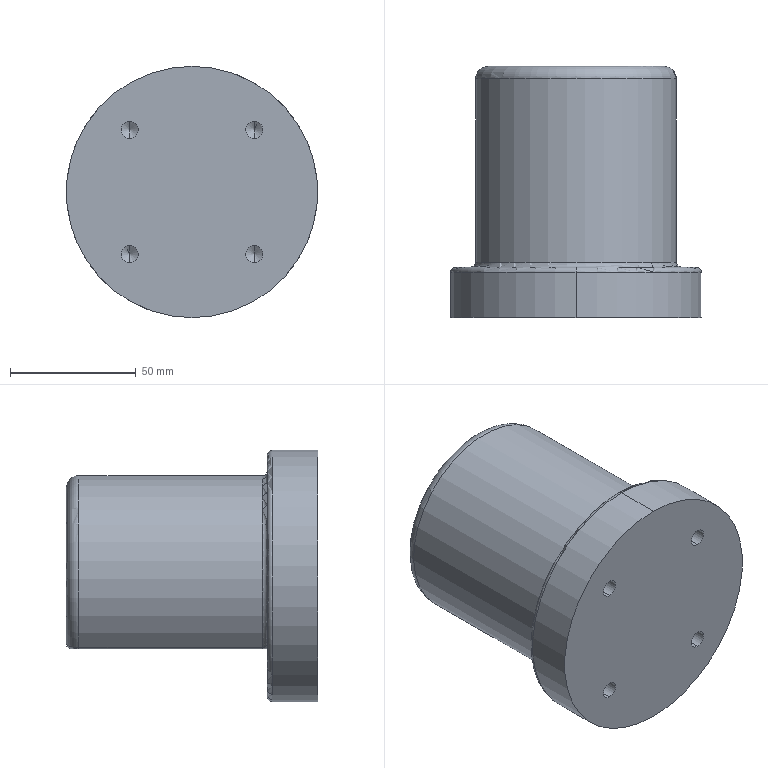Part | STEP file | Tube-changer group fixed foot (threading) SGN-2-14-02 | 1 solid | 45 faces | box 100 x 100 x 100 mm | volume 484846 mm3 | cylinder 18 | plane 11 | cone 8 | torus 4 | spline 4 | commonest cylinder face diameters 6.8 x8 4 x3 30 x2 40 x2 100 x2 80 x1